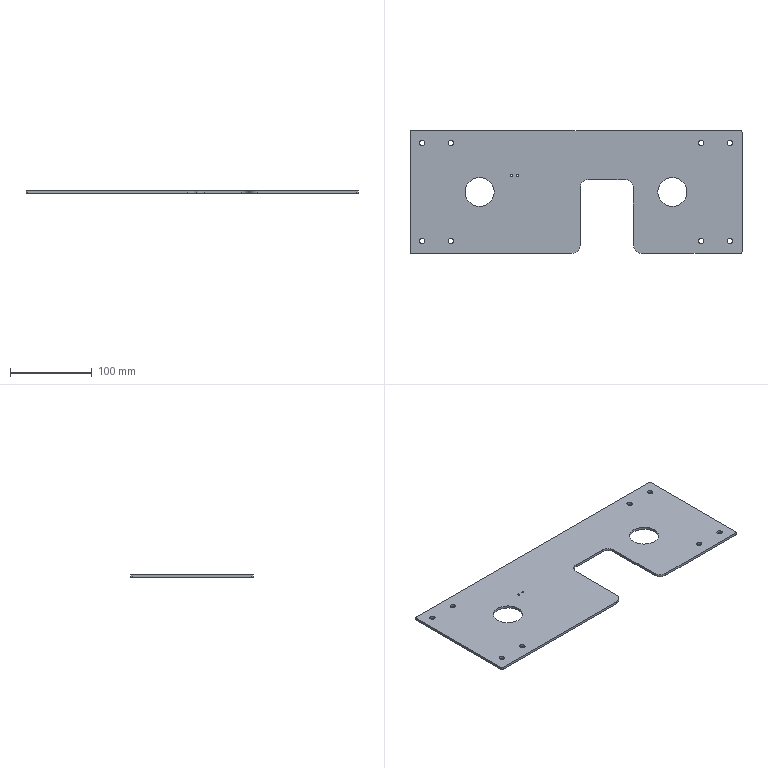Part | STEP file | Bottom adapter plate | 1 solid | 42 faces | box 405 x 150 x 3 mm | volume 157925 mm3 | cylinder 32 | plane 10 | commonest cylinder face diameters 6.5 x16 2.5 x4 4 x4 20 x4 35.5 x4